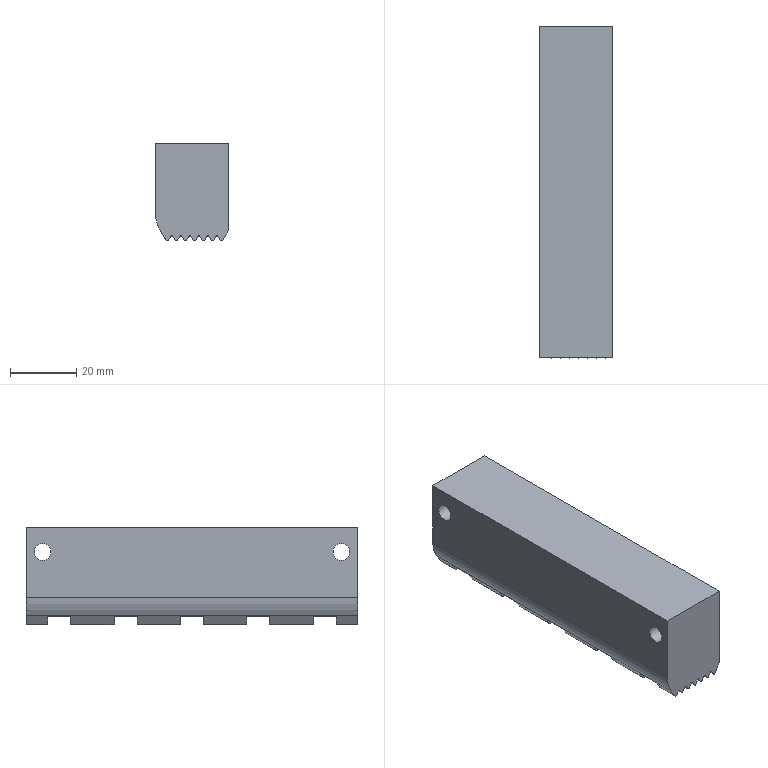Part | STEP file | 1 solid | 175 faces | box 22 x 100 x 29.5 mm | volume 60333 mm3 | plane 94 | cylinder 81 | commonest cylinder face diameters 0.68 x42 0.72 x36 5.02 x2 20 x1